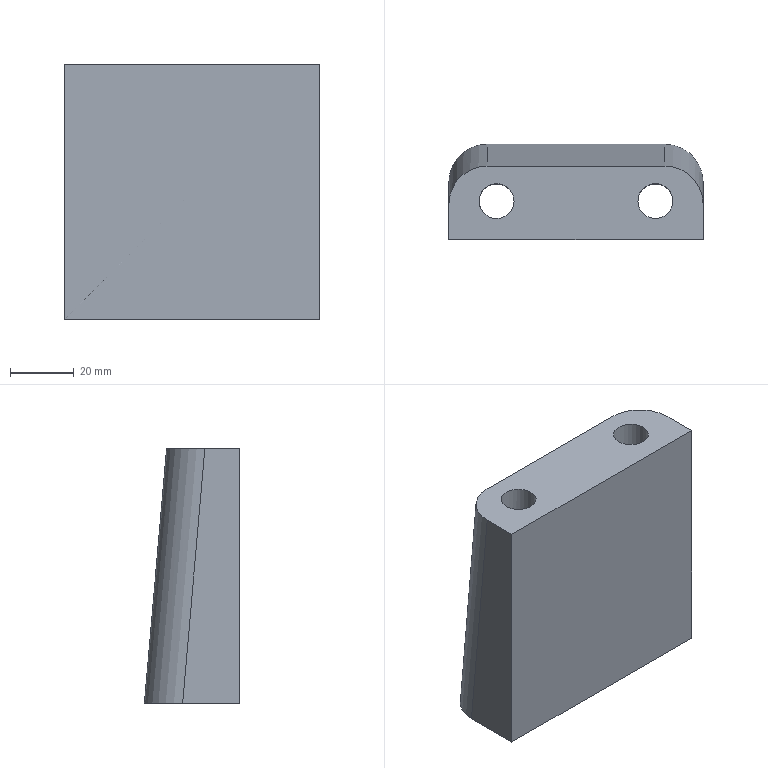Part | STEP file | solid 124 | 1 solid | 18 faces | box 80 x 30 x 80 mm | volume 143867 mm3 | plane 8 | cylinder 8 | cone 2 | commonest cylinder face diameters 11 x2 18 x2 24 x2 9 x1 10 x1